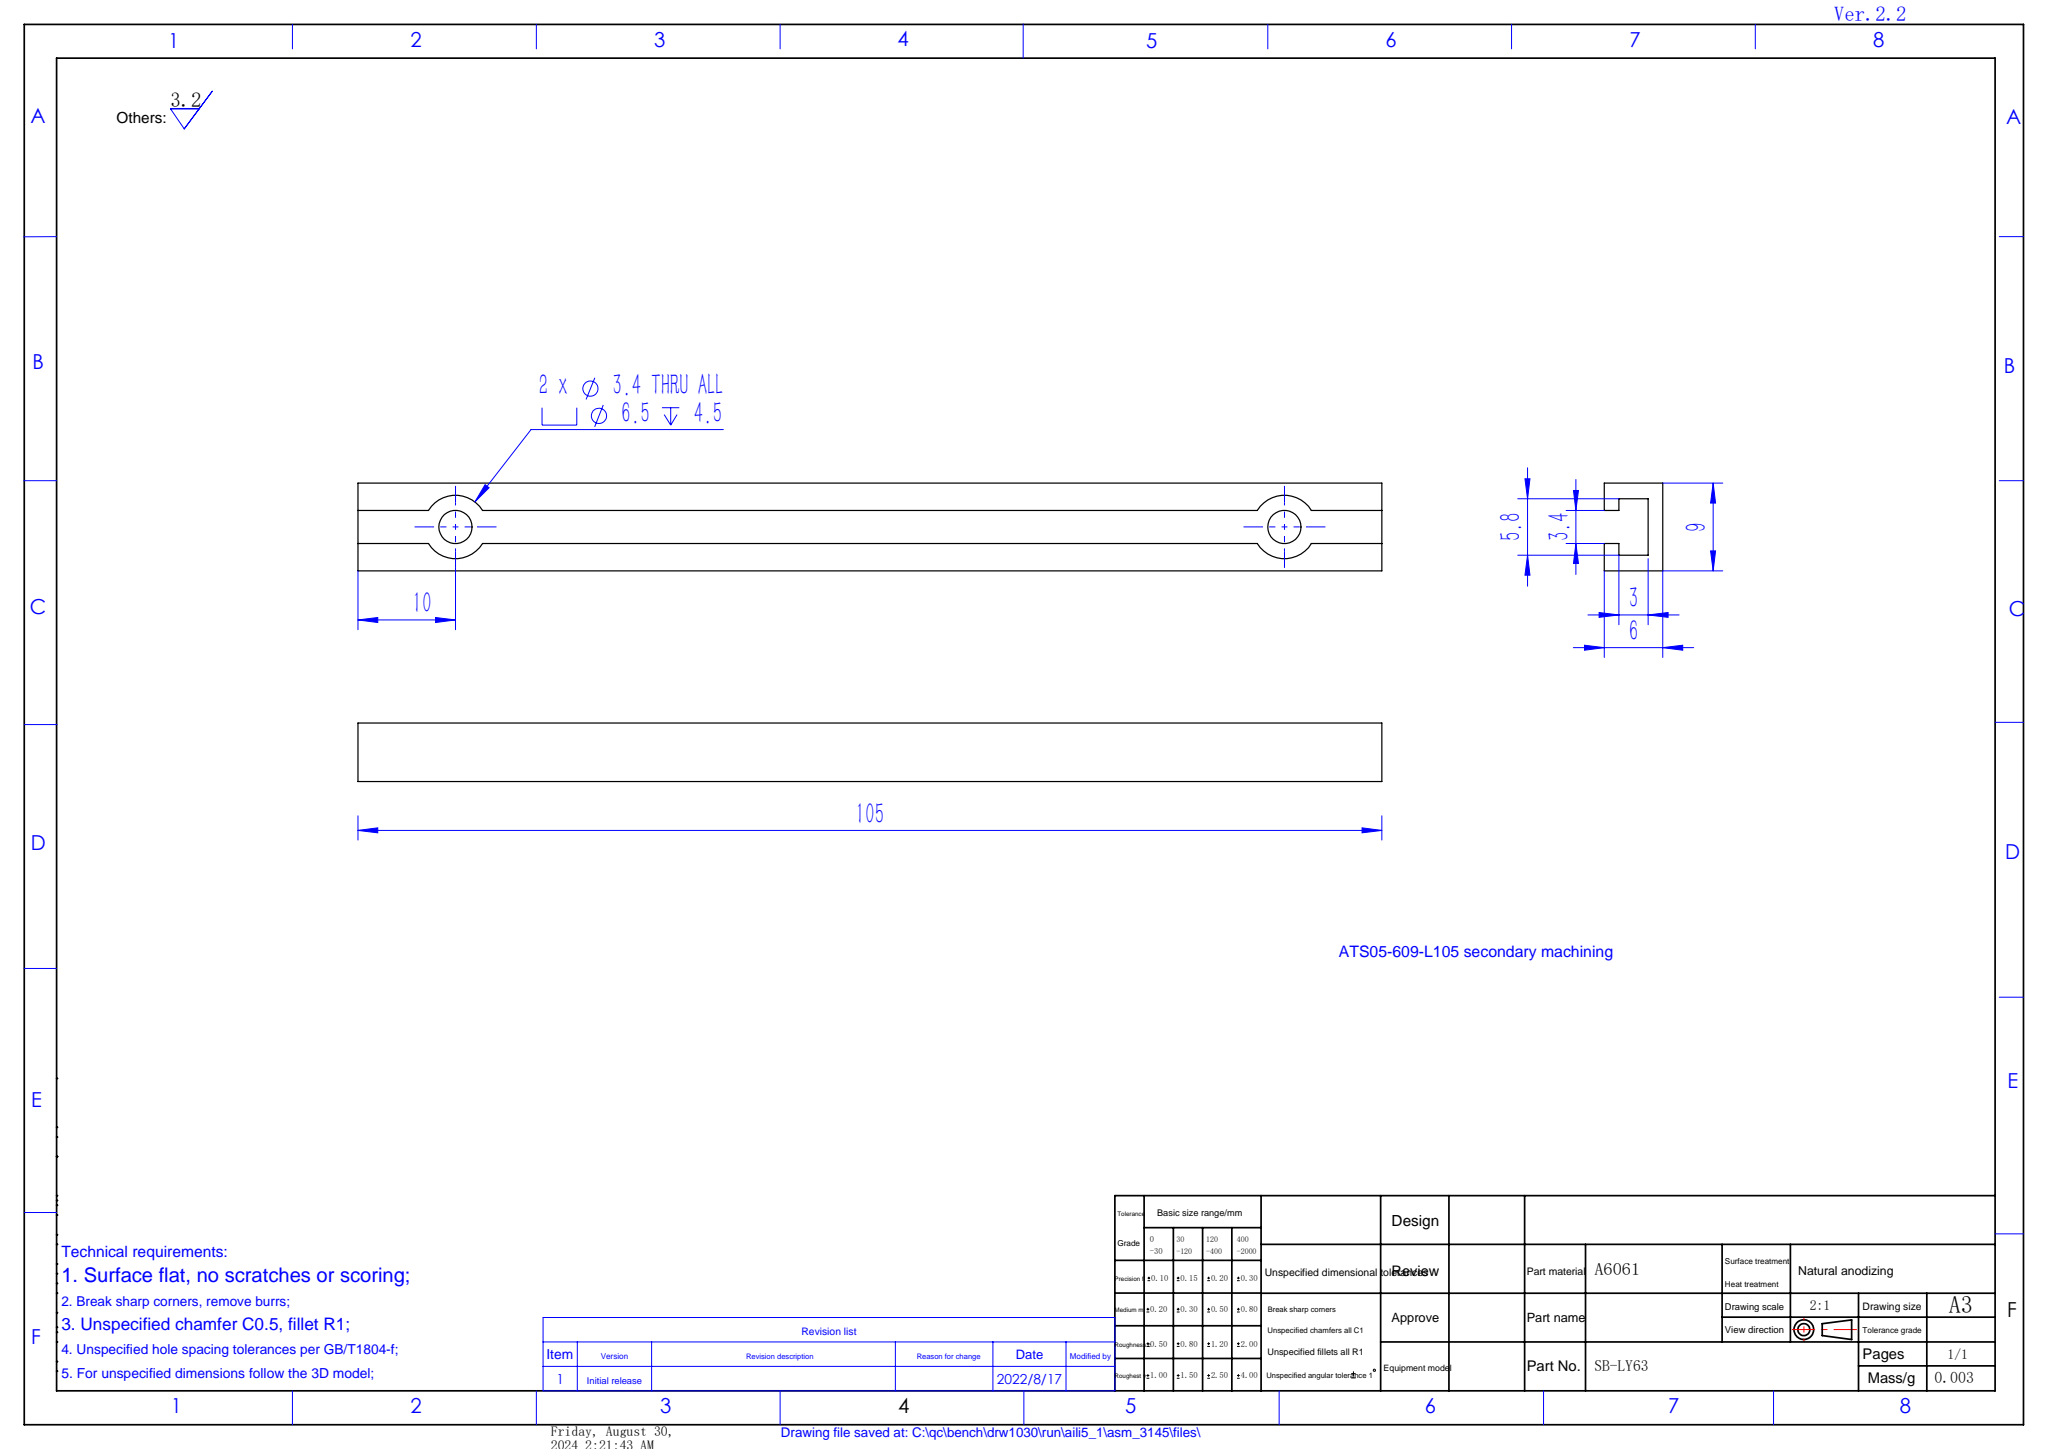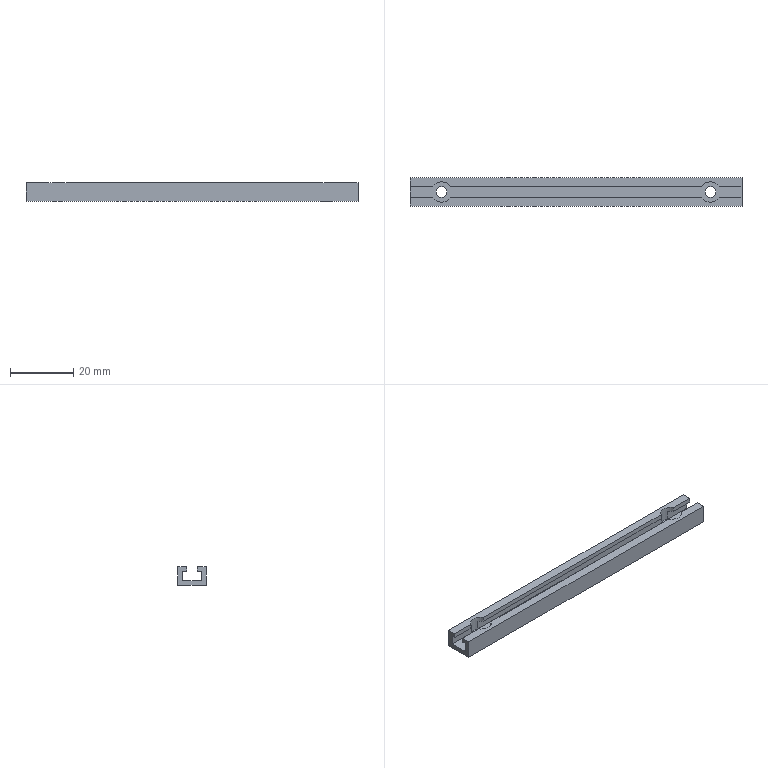Part | SolidWorks | features ICE 2, BaseBody 1, Cut 1, HoleWzd 1, MoveFace 1 | 1 solid | 34 faces | box 105 x 9 x 6 mm | volume 3236 mm3 | plane 26 | cylinder 8 | commonest cylinder face diameters 3.4 x4 6.5 x4